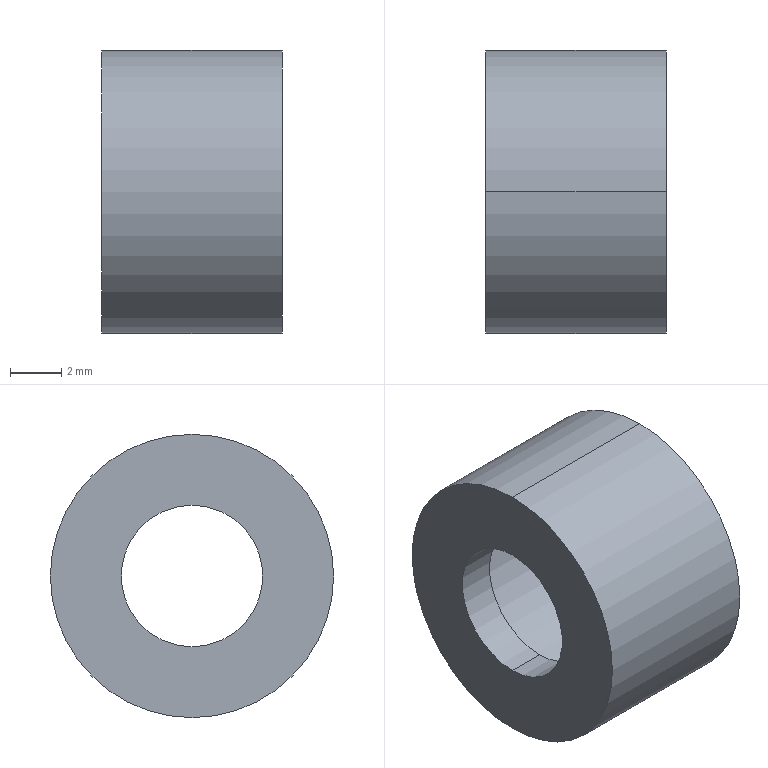Part | SolidWorks | features Extrusion 1, ICE 1 | 1 solid | 9 faces | box 7 x 11 x 11 mm | volume 317.497 mm3 | cylinder 6 | plane 3 | commonest cylinder face diameters 5.5 x2 8.5 x2 11 x2
STEP:
#1=CARTESIAN_POINT('',(1.5,0.,4.25));
#2=VERTEX_POINT('',#1);
#3=CARTESIAN_POINT('',(1.5,0.,-4.25));
#4=VERTEX_POINT('',#3);
#5=CARTESIAN_POINT('',(1.5,0.,0.));
#6=DIRECTION('',(1.,0.,0.));
#7=DIRECTION('',(0.,0.,-1.));
#8=AXIS2_PLACEMENT_3D('',#5,#6,#7);
#9=CIRCLE('',#8,4.25);
#10=EDGE_CURVE('',#2,#4,#9,.T.);
#11=ORIENTED_EDGE('',*,*,#10,.F.);
#12=CARTESIAN_POINT('',(7.,0.,4.25));
#13=VERTEX_POINT('',#12);
#14=CARTESIAN_POINT('',(1.5,0.,4.25));
#15=DIRECTION('',(1.,0.,0.));
#16=VECTOR('',#15,1000.);
#17=LINE('',#14,#16);
#18=EDGE_CURVE('',#2,#13,#17,.T.);
#19=ORIENTED_EDGE('',*,*,#18,.T.);
#20=CARTESIAN_POINT('',(7.,0.,-4.25));
#21=VERTEX_POINT('',#20);
#22=CARTESIAN_POINT('',(7.,0.,0.));
#23=DIRECTION('',(1.,0.,0.));
#24=DIRECTION('',(0.,0.,-1.));
#25=AXIS2_PLACEMENT_3D('',#22,#23,#24);
#26=CIRCLE('',#25,4.25);
#27=EDGE_CURVE('',#13,#21,#26,.T.);
#28=ORIENTED_EDGE('',*,*,#27,.T.);
#29=CARTESIAN_POINT('',(1.5,0.,-4.25));
#30=DIRECTION('',(1.,0.,0.));
#31=VECTOR('',#30,1000.);
#32=LINE('',#29,#31);
#33=EDGE_CURVE('',#4,#21,#32,.T.);
#34=ORIENTED_EDGE('',*,*,#33,.F.);
#35=EDGE_LOOP('',(#11,#19,#28,#34));
#36=FACE_OUTER_BOUND('',#35,.T.);
#37=CARTESIAN_POINT('',(1.5,0.,0.));
#38=DIRECTION('',(1.,0.,0.));
#39=DIRECTION('',(0.,0.,-1.));
#40=AXIS2_PLACEMENT_3D('',#37,#38,#39);
#41=CYLINDRICAL_SURFACE('',#40,4.25);
#42=ADVANCED_FACE('',(#36),#41,.F.);
#43=CARTESIAN_POINT('',(7.,0.,-5.5));
#44=VERTEX_POINT('',#43);
#45=CARTESIAN_POINT('',(7.,0.,5.5));
#46=VERTEX_POINT('',#45);
#47=CARTESIAN_POINT('',(7.,0.,0.));
#48=DIRECTION('',(1.,0.,0.));
#49=DIRECTION('',(0.,0.,-1.));
#50=AXIS2_PLACEMENT_3D('',#47,#48,#49);
#51=CIRCLE('',#50,5.5);
#52=EDGE_CURVE('',#44,#46,#51,.T.);
#53=ORIENTED_EDGE('',*,*,#52,.F.);
#54=CARTESIAN_POINT('',(0.,0.,-5.5));
#55=VERTEX_POINT('',#54);
#56=CARTESIAN_POINT('',(7.,0.,-5.5));
#57=DIRECTION('',(-1.,0.,0.));
#58=VECTOR('',#57,1000.);
#59=LINE('',#56,#58);
#60=EDGE_CURVE('',#44,#55,#59,.T.);
#61=ORIENTED_EDGE('',*,*,#60,.T.);
#62=CARTESIAN_POINT('',(0.,0.,5.5));
#63=VERTEX_POINT('',#62);
#64=CARTESIAN_POINT('',(0.,0.,0.));
#65=DIRECTION('',(1.,0.,0.));
#66=DIRECTION('',(0.,0.,-1.));
#67=AXIS2_PLACEMENT_3D('',#64,#65,#66);
#68=CIRCLE('',#67,5.5);
#69=EDGE_CURVE('',#55,#63,#68,.T.);
#70=ORIENTED_EDGE('',*,*,#69,.T.);
#71=CARTESIAN_POINT('',(7.,0.,5.5));
#72=DIRECTION('',(-1.,0.,0.));
#73=VECTOR('',#72,1000.);
#74=LINE('',#71,#73);
#75=EDGE_CURVE('',#46,#63,#74,.T.);
#76=ORIENTED_EDGE('',*,*,#75,.F.);
#77=EDGE_LOOP('',(#53,#61,#70,#76));
#78=FACE_OUTER_BOUND('',#77,.T.);
#79=CARTESIAN_POINT('',(7.,0.,0.));
#80=DIRECTION('',(-1.,0.,0.));
#81=DIRECTION('',(0.,0.,1.));
#82=AXIS2_PLACEMENT_3D('',#79,#80,#81);
#83=CYLINDRICAL_SURFACE('',#82,5.5);
#84=ADVANCED_FACE('',(#78),#83,.T.);
#85=CARTESIAN_POINT('',(1.5,0.,2.75));
#86=VERTEX_POINT('',#85);
#87=CARTESIAN_POINT('',(1.5,0.,-2.75));
#88=VERTEX_POINT('',#87);
#89=CARTESIAN_POINT('',(1.5,0.,0.));
#90=DIRECTION('',(1.,0.,0.));
#91=DIRECTION('',(0.,0.,-1.));
#92=AXIS2_PLACEMENT_3D('',#89,#90,#91);
#93=CIRCLE('',#92,2.75);
#94=EDGE_CURVE('',#86,#88,#93,.T.);
#95=ORIENTED_EDGE('',*,*,#94,.T.);
#96=CARTESIAN_POINT('',(0.,0.,-2.75));
#97=VERTEX_POINT('',#96);
#98=CARTESIAN_POINT('',(7.,0.,-2.75));
#99=DIRECTION('',(-1.,0.,0.));
#100=VECTOR('',#99,1000.);
#101=LINE('',#98,#100);
#102=EDGE_CURVE('',#88,#97,#101,.T.);
#103=ORIENTED_EDGE('',*,*,#102,.T.);
#104=CARTESIAN_POINT('',(0.,0.,2.75));
#105=VERTEX_POINT('',#104);
#106=CARTESIAN_POINT('',(0.,0.,0.));
#107=DIRECTION('',(1.,0.,0.));
#108=DIRECTION('',(0.,0.,-1.));
#109=AXIS2_PLACEMENT_3D('',#106,#107,#108);
#110=CIRCLE('',#109,2.75);
#111=EDGE_CURVE('',#105,#97,#110,.T.);
#112=ORIENTED_EDGE('',*,*,#111,.F.);
#113=CARTESIAN_POINT('',(7.,0.,2.75));
#114=DIRECTION('',(-1.,0.,0.));
#115=VECTOR('',#114,1000.);
#116=LINE('',#113,#115);
#117=EDGE_CURVE('',#86,#105,#116,.T.);
#118=ORIENTED_EDGE('',*,*,#117,.F.);
#119=EDGE_LOOP('',(#95,#103,#112,#118));
#120=FACE_OUTER_BOUND('',#119,.T.);
#121=CARTESIAN_POINT('',(7.,0.,0.));
#122=DIRECTION('',(-1.,0.,0.));
#123=DIRECTION('',(0.,0.,1.));
#124=AXIS2_PLACEMENT_3D('',#121,#122,#123);
#125=CYLINDRICAL_SURFACE('',#124,2.75);
#126=ADVANCED_FACE('',(#120),#125,.F.);
#127=ORIENTED_EDGE('',*,*,#102,.F.);
#128=CARTESIAN_POINT('',(1.5,0.,0.));
#129=DIRECTION('',(1.,0.,0.));
#130=DIRECTION('',(0.,0.,-1.));
#131=AXIS2_PLACEMENT_3D('',#128,#129,#130);
#132=CIRCLE('',#131,2.75);
#133=EDGE_CURVE('',#88,#86,#132,.T.);
#134=ORIENTED_EDGE('',*,*,#133,.T.);
#135=ORIENTED_EDGE('',*,*,#117,.T.);
#136=CARTESIAN_POINT('',(0.,0.,0.));
#137=DIRECTION('',(1.,0.,0.));
#138=DIRECTION('',(0.,0.,-1.));
#139=AXIS2_PLACEMENT_3D('',#136,#137,#138);
#140=CIRCLE('',#139,2.75);
#141=EDGE_CURVE('',#97,#105,#140,.T.);
#142=ORIENTED_EDGE('',*,*,#141,.F.);
#143=EDGE_LOOP('',(#127,#134,#135,#142));
#144=FACE_OUTER_BOUND('',#143,.T.);
#145=CARTESIAN_POINT('',(7.,0.,0.));
#146=DIRECTION('',(-1.,0.,0.));
#147=DIRECTION('',(0.,0.,1.));
#148=AXIS2_PLACEMENT_3D('',#145,#146,#147);
#149=CYLINDRICAL_SURFACE('',#148,2.75);
#150=ADVANCED_FACE('',(#144),#149,.F.);
#151=CARTESIAN_POINT('',(7.,0.,0.));
#152=DIRECTION('',(1.,0.,0.));
#153=DIRECTION('',(0.,0.,-1.));
#154=AXIS2_PLACEMENT_3D('',#151,#152,#153);
#155=CIRCLE('',#154,4.25);
#156=EDGE_CURVE('',#21,#13,#155,.T.);
#157=ORIENTED_EDGE('',*,*,#156,.F.);
#158=ORIENTED_EDGE('',*,*,#27,.F.);
#159=EDGE_LOOP('',(#157,#158));
#160=FACE_BOUND('',#159,.T.);
#161=CARTESIAN_POINT('',(7.,0.,0.));
#162=DIRECTION('',(1.,0.,0.));
#163=DIRECTION('',(0.,0.,-1.));
#164=AXIS2_PLACEMENT_3D('',#161,#162,#163);
#165=CIRCLE('',#164,5.5);
#166=EDGE_CURVE('',#46,#44,#165,.T.);
#167=ORIENTED_EDGE('',*,*,#166,.T.);
#168=ORIENTED_EDGE('',*,*,#52,.T.);
#169=EDGE_LOOP('',(#167,#168));
#170=FACE_OUTER_BOUND('',#169,.T.);
#171=CARTESIAN_POINT('',(7.,0.,0.));
#172=DIRECTION('',(1.,0.,0.));
#173=DIRECTION('',(0.,0.,-1.));
#174=AXIS2_PLACEMENT_3D('',#171,#172,#173);
#175=PLANE('',#174);
#176=ADVANCED_FACE('',(#160,#170),#175,.T.);
#177=CARTESIAN_POINT('',(0.,0.,0.));
#178=DIRECTION('',(1.,0.,0.));
#179=DIRECTION('',(0.,0.,-1.));
#180=AXIS2_PLACEMENT_3D('',#177,#178,#179);
#181=CIRCLE('',#180,5.5);
#182=EDGE_CURVE('',#63,#55,#181,.T.);
#183=ORIENTED_EDGE('',*,*,#182,.F.);
#184=ORIENTED_EDGE('',*,*,#69,.F.);
#185=EDGE_LOOP('',(#183,#184));
#186=FACE_OUTER_BOUND('',#185,.T.);
#187=ORIENTED_EDGE('',*,*,#111,.T.);
#188=ORIENTED_EDGE('',*,*,#141,.T.);
#189=EDGE_LOOP('',(#187,#188));
#190=FACE_BOUND('',#189,.T.);
#191=CARTESIAN_POINT('',(0.,0.,0.));
#192=DIRECTION('',(1.,0.,0.));
#193=DIRECTION('',(0.,0.,-1.));
#194=AXIS2_PLACEMENT_3D('',#191,#192,#193);
#195=PLANE('',#194);
#196=ADVANCED_FACE('',(#186,#190),#195,.F.);
#197=ORIENTED_EDGE('',*,*,#60,.F.);
#198=ORIENTED_EDGE('',*,*,#166,.F.);
#199=ORIENTED_EDGE('',*,*,#75,.T.);
#200=ORIENTED_EDGE('',*,*,#182,.T.);
#201=EDGE_LOOP('',(#197,#198,#199,#200));
#202=FACE_OUTER_BOUND('',#201,.T.);
#203=CARTESIAN_POINT('',(7.,0.,0.));
#204=DIRECTION('',(-1.,0.,0.));
#205=DIRECTION('',(0.,0.,1.));
#206=AXIS2_PLACEMENT_3D('',#203,#204,#205);
#207=CYLINDRICAL_SURFACE('',#206,5.5);
#208=ADVANCED_FACE('',(#202),#207,.T.);
#209=ORIENTED_EDGE('',*,*,#18,.F.);
#210=CARTESIAN_POINT('',(1.5,0.,0.));
#211=DIRECTION('',(1.,0.,0.));
#212=DIRECTION('',(0.,0.,-1.));
#213=AXIS2_PLACEMENT_3D('',#210,#211,#212);
#214=CIRCLE('',#213,4.25);
#215=EDGE_CURVE('',#4,#2,#214,.T.);
#216=ORIENTED_EDGE('',*,*,#215,.F.);
#217=ORIENTED_EDGE('',*,*,#33,.T.);
#218=ORIENTED_EDGE('',*,*,#156,.T.);
#219=EDGE_LOOP('',(#209,#216,#217,#218));
#220=FACE_OUTER_BOUND('',#219,.T.);
#221=CARTESIAN_POINT('',(1.5,0.,0.));
#222=DIRECTION('',(1.,0.,0.));
#223=DIRECTION('',(0.,0.,-1.));
#224=AXIS2_PLACEMENT_3D('',#221,#222,#223);
#225=CYLINDRICAL_SURFACE('',#224,4.25);
#226=ADVANCED_FACE('',(#220),#225,.F.);
#227=ORIENTED_EDGE('',*,*,#94,.F.);
#228=ORIENTED_EDGE('',*,*,#133,.F.);
#229=EDGE_LOOP('',(#227,#228));
#230=FACE_BOUND('',#229,.T.);
#231=ORIENTED_EDGE('',*,*,#215,.T.);
#232=ORIENTED_EDGE('',*,*,#10,.T.);
#233=EDGE_LOOP('',(#231,#232));
#234=FACE_OUTER_BOUND('',#233,.T.);
#235=CARTESIAN_POINT('',(1.5,0.,0.));
#236=DIRECTION('',(1.,0.,0.));
#237=DIRECTION('',(0.,0.,-1.));
#238=AXIS2_PLACEMENT_3D('',#235,#236,#237);
#239=PLANE('',#238);
#240=ADVANCED_FACE('',(#230,#234),#239,.T.);
#241=CLOSED_SHELL('',(#42,#84,#126,#150,#176,#196,#208,#226,#240));
#242=MANIFOLD_SOLID_BREP('',#241);
#243=CARTESIAN_POINT('',(0.,0.,0.));
#244=DIRECTION('',(0.,0.,1.));
#245=DIRECTION('',(1.,0.,0.));
#246=AXIS2_PLACEMENT_3D('',#243,#244,#245);
#247=(LENGTH_UNIT()NAMED_UNIT(*)SI_UNIT(.MILLI.,.METRE.));
#248=UNCERTAINTY_MEASURE_WITH_UNIT(LENGTH_MEASURE(0.00001),#247,'','');
#249=(NAMED_UNIT(*)PLANE_ANGLE_UNIT()SI_UNIT($,.RADIAN.));
#250=(NAMED_UNIT(*)SI_UNIT($,.STERADIAN.)SOLID_ANGLE_UNIT());
#251=(GEOMETRIC_REPRESENTATION_CONTEXT(3)GLOBAL_UNCERTAINTY_ASSIGNED_CONTEXT((#248))GLOBAL_UNIT_ASSIGNED_CONTEXT((#247,#249,#250))REPRESENTATION_CONTEXT('',''));
#252=ADVANCED_BREP_SHAPE_REPRESENTATION('',(#242,#246),#251);